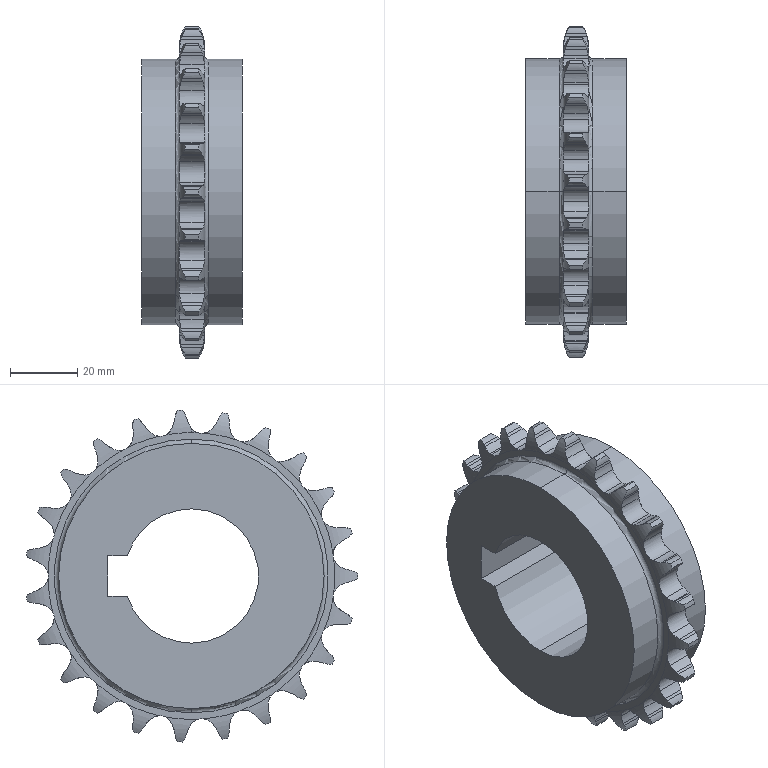Part | SolidWorks | features ICE 2, CirPattern 1, Cut 1, RefAxis 1, Revolution 1 | 1 solid | 262 faces | box 30 x 98.633 x 98.858 mm | volume 118578 mm3 | cylinder 157 | plane 53 | torus 52 | commonest cylinder face diameters 11.437 x49 20.732 x48 8.06 x30 99 x23 79 x4 40 x3